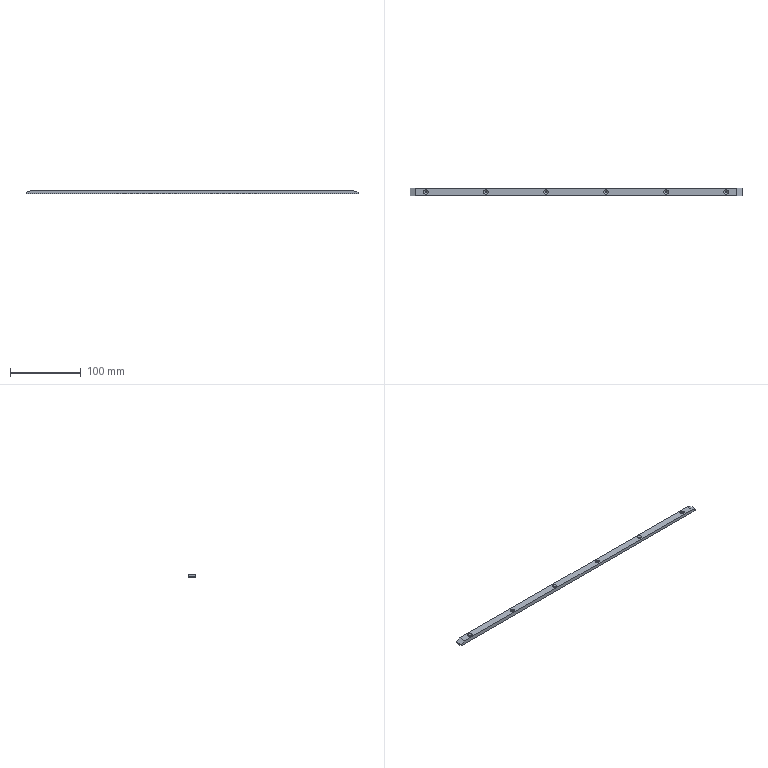Part | NX | features BREP 1 | 1 solid | 32 faces | box 470 x 10 x 5 mm | volume 22916 mm3 | cone 12 | cylinder 12 | plane 8 | commonest cylinder face diameters 3.4 x12
STEP:
#1=CARTESIAN_POINT('',(-215.65,0.,5.));
#2=VERTEX_POINT('',#1);
#3=CARTESIAN_POINT('',(-214.2,0.,3.55));
#4=VERTEX_POINT('',#3);
#5=CARTESIAN_POINT('',(-215.65,0.,5.));
#6=DIRECTION('',(-0.7071,0.,0.7071));
#7=VECTOR('',#6,1000.);
#8=LINE('',#5,#7);
#9=EDGE_CURVE('',#2,#4,#8,.F.);
#10=ORIENTED_EDGE('',*,*,#9,.T.);
#11=CARTESIAN_POINT('',(-210.8,0.,3.55));
#12=VERTEX_POINT('',#11);
#13=CARTESIAN_POINT('',(-212.5,0.,3.55));
#14=DIRECTION('',(0.,0.,1.));
#15=DIRECTION('',(1.,0.,0.));
#16=AXIS2_PLACEMENT_3D('',#13,#14,#15);
#17=CIRCLE('',#16,1.7);
#18=EDGE_CURVE('',#12,#4,#17,.T.);
#19=ORIENTED_EDGE('',*,*,#18,.F.);
#20=CARTESIAN_POINT('',(-209.35,0.,5.));
#21=VERTEX_POINT('',#20);
#22=CARTESIAN_POINT('',(-209.35,0.,5.));
#23=DIRECTION('',(0.7071,0.,0.7071));
#24=VECTOR('',#23,1000.);
#25=LINE('',#22,#24);
#26=EDGE_CURVE('',#21,#12,#25,.F.);
#27=ORIENTED_EDGE('',*,*,#26,.F.);
#28=CARTESIAN_POINT('',(-212.5,0.,5.));
#29=DIRECTION('',(0.,0.,1.));
#30=DIRECTION('',(1.,0.,0.));
#31=AXIS2_PLACEMENT_3D('',#28,#29,#30);
#32=CIRCLE('',#31,3.15);
#33=EDGE_CURVE('',#21,#2,#32,.T.);
#34=ORIENTED_EDGE('',*,*,#33,.T.);
#35=EDGE_LOOP('',(#10,#19,#27,#34));
#36=FACE_BOUND('',#35,.T.);
#37=CARTESIAN_POINT('',(-212.5,0.,5.));
#38=DIRECTION('',(0.,0.,1.));
#39=DIRECTION('',(1.,0.,0.));
#40=AXIS2_PLACEMENT_3D('',#37,#38,#39);
#41=CONICAL_SURFACE('',#40,3.15,0.7854);
#42=ADVANCED_FACE('',(#36),#41,.F.);
#43=CARTESIAN_POINT('',(-214.2,0.,0.));
#44=VERTEX_POINT('',#43);
#45=CARTESIAN_POINT('',(-214.2,0.,5.));
#46=DIRECTION('',(0.,0.,1.));
#47=VECTOR('',#46,1000.);
#48=LINE('',#45,#47);
#49=EDGE_CURVE('',#4,#44,#48,.F.);
#50=ORIENTED_EDGE('',*,*,#49,.T.);
#51=CARTESIAN_POINT('',(-210.8,0.,0.));
#52=VERTEX_POINT('',#51);
#53=CARTESIAN_POINT('',(-212.5,0.,0.));
#54=DIRECTION('',(0.,0.,1.));
#55=DIRECTION('',(1.,0.,0.));
#56=AXIS2_PLACEMENT_3D('',#53,#54,#55);
#57=CIRCLE('',#56,1.7);
#58=EDGE_CURVE('',#52,#44,#57,.T.);
#59=ORIENTED_EDGE('',*,*,#58,.F.);
#60=CARTESIAN_POINT('',(-210.8,0.,5.));
#61=DIRECTION('',(0.,0.,1.));
#62=VECTOR('',#61,1000.);
#63=LINE('',#60,#62);
#64=EDGE_CURVE('',#12,#52,#63,.F.);
#65=ORIENTED_EDGE('',*,*,#64,.F.);
#66=ORIENTED_EDGE('',*,*,#18,.T.);
#67=EDGE_LOOP('',(#50,#59,#65,#66));
#68=FACE_BOUND('',#67,.T.);
#69=CARTESIAN_POINT('',(-212.5,0.,5.));
#70=DIRECTION('',(0.,0.,1.));
#71=DIRECTION('',(1.,0.,0.));
#72=AXIS2_PLACEMENT_3D('',#69,#70,#71);
#73=CYLINDRICAL_SURFACE('',#72,1.7);
#74=ADVANCED_FACE('',(#68),#73,.F.);
#75=CARTESIAN_POINT('',(-130.65,0.,5.));
#76=VERTEX_POINT('',#75);
#77=CARTESIAN_POINT('',(-129.2,0.,3.55));
#78=VERTEX_POINT('',#77);
#79=CARTESIAN_POINT('',(-130.65,0.,5.));
#80=DIRECTION('',(-0.7071,0.,0.7071));
#81=VECTOR('',#80,1000.);
#82=LINE('',#79,#81);
#83=EDGE_CURVE('',#76,#78,#82,.F.);
#84=ORIENTED_EDGE('',*,*,#83,.T.);
#85=CARTESIAN_POINT('',(-125.8,0.,3.55));
#86=VERTEX_POINT('',#85);
#87=CARTESIAN_POINT('',(-127.5,0.,3.55));
#88=DIRECTION('',(0.,0.,1.));
#89=DIRECTION('',(1.,0.,0.));
#90=AXIS2_PLACEMENT_3D('',#87,#88,#89);
#91=CIRCLE('',#90,1.7);
#92=EDGE_CURVE('',#86,#78,#91,.T.);
#93=ORIENTED_EDGE('',*,*,#92,.F.);
#94=CARTESIAN_POINT('',(-124.35,0.,5.));
#95=VERTEX_POINT('',#94);
#96=CARTESIAN_POINT('',(-124.35,0.,5.));
#97=DIRECTION('',(0.7071,0.,0.7071));
#98=VECTOR('',#97,1000.);
#99=LINE('',#96,#98);
#100=EDGE_CURVE('',#95,#86,#99,.F.);
#101=ORIENTED_EDGE('',*,*,#100,.F.);
#102=CARTESIAN_POINT('',(-127.5,0.,5.));
#103=DIRECTION('',(0.,0.,1.));
#104=DIRECTION('',(1.,0.,0.));
#105=AXIS2_PLACEMENT_3D('',#102,#103,#104);
#106=CIRCLE('',#105,3.15);
#107=EDGE_CURVE('',#95,#76,#106,.T.);
#108=ORIENTED_EDGE('',*,*,#107,.T.);
#109=EDGE_LOOP('',(#84,#93,#101,#108));
#110=FACE_BOUND('',#109,.T.);
#111=CARTESIAN_POINT('',(-127.5,0.,5.));
#112=DIRECTION('',(0.,0.,1.));
#113=DIRECTION('',(1.,0.,0.));
#114=AXIS2_PLACEMENT_3D('',#111,#112,#113);
#115=CONICAL_SURFACE('',#114,3.15,0.7854);
#116=ADVANCED_FACE('',(#110),#115,.F.);
#117=CARTESIAN_POINT('',(-129.2,0.,0.));
#118=VERTEX_POINT('',#117);
#119=CARTESIAN_POINT('',(-129.2,0.,5.));
#120=DIRECTION('',(0.,0.,1.));
#121=VECTOR('',#120,1000.);
#122=LINE('',#119,#121);
#123=EDGE_CURVE('',#78,#118,#122,.F.);
#124=ORIENTED_EDGE('',*,*,#123,.T.);
#125=CARTESIAN_POINT('',(-125.8,0.,0.));
#126=VERTEX_POINT('',#125);
#127=CARTESIAN_POINT('',(-127.5,0.,0.));
#128=DIRECTION('',(0.,0.,1.));
#129=DIRECTION('',(1.,0.,0.));
#130=AXIS2_PLACEMENT_3D('',#127,#128,#129);
#131=CIRCLE('',#130,1.7);
#132=EDGE_CURVE('',#126,#118,#131,.T.);
#133=ORIENTED_EDGE('',*,*,#132,.F.);
#134=CARTESIAN_POINT('',(-125.8,0.,5.));
#135=DIRECTION('',(0.,0.,1.));
#136=VECTOR('',#135,1000.);
#137=LINE('',#134,#136);
#138=EDGE_CURVE('',#86,#126,#137,.F.);
#139=ORIENTED_EDGE('',*,*,#138,.F.);
#140=ORIENTED_EDGE('',*,*,#92,.T.);
#141=EDGE_LOOP('',(#124,#133,#139,#140));
#142=FACE_BOUND('',#141,.T.);
#143=CARTESIAN_POINT('',(-127.5,0.,5.));
#144=DIRECTION('',(0.,0.,1.));
#145=DIRECTION('',(1.,0.,0.));
#146=AXIS2_PLACEMENT_3D('',#143,#144,#145);
#147=CYLINDRICAL_SURFACE('',#146,1.7);
#148=ADVANCED_FACE('',(#142),#147,.F.);
#149=CARTESIAN_POINT('',(-45.65,0.,5.));
#150=VERTEX_POINT('',#149);
#151=CARTESIAN_POINT('',(-44.2,0.,3.55));
#152=VERTEX_POINT('',#151);
#153=CARTESIAN_POINT('',(-45.65,0.,5.));
#154=DIRECTION('',(-0.7071,0.,0.7071));
#155=VECTOR('',#154,1000.);
#156=LINE('',#153,#155);
#157=EDGE_CURVE('',#150,#152,#156,.F.);
#158=ORIENTED_EDGE('',*,*,#157,.T.);
#159=CARTESIAN_POINT('',(-40.8,0.,3.55));
#160=VERTEX_POINT('',#159);
#161=CARTESIAN_POINT('',(-42.5,0.,3.55));
#162=DIRECTION('',(0.,0.,1.));
#163=DIRECTION('',(1.,0.,0.));
#164=AXIS2_PLACEMENT_3D('',#161,#162,#163);
#165=CIRCLE('',#164,1.7);
#166=EDGE_CURVE('',#160,#152,#165,.T.);
#167=ORIENTED_EDGE('',*,*,#166,.F.);
#168=CARTESIAN_POINT('',(-39.35,0.,5.));
#169=VERTEX_POINT('',#168);
#170=CARTESIAN_POINT('',(-39.35,0.,5.));
#171=DIRECTION('',(0.7071,0.,0.7071));
#172=VECTOR('',#171,1000.);
#173=LINE('',#170,#172);
#174=EDGE_CURVE('',#169,#160,#173,.F.);
#175=ORIENTED_EDGE('',*,*,#174,.F.);
#176=CARTESIAN_POINT('',(-42.5,0.,5.));
#177=DIRECTION('',(0.,0.,1.));
#178=DIRECTION('',(1.,0.,0.));
#179=AXIS2_PLACEMENT_3D('',#176,#177,#178);
#180=CIRCLE('',#179,3.15);
#181=EDGE_CURVE('',#169,#150,#180,.T.);
#182=ORIENTED_EDGE('',*,*,#181,.T.);
#183=EDGE_LOOP('',(#158,#167,#175,#182));
#184=FACE_BOUND('',#183,.T.);
#185=CARTESIAN_POINT('',(-42.5,0.,5.));
#186=DIRECTION('',(0.,0.,1.));
#187=DIRECTION('',(1.,0.,0.));
#188=AXIS2_PLACEMENT_3D('',#185,#186,#187);
#189=CONICAL_SURFACE('',#188,3.15,0.7854);
#190=ADVANCED_FACE('',(#184),#189,.F.);
#191=CARTESIAN_POINT('',(-44.2,0.,0.));
#192=VERTEX_POINT('',#191);
#193=CARTESIAN_POINT('',(-44.2,0.,5.));
#194=DIRECTION('',(0.,0.,1.));
#195=VECTOR('',#194,1000.);
#196=LINE('',#193,#195);
#197=EDGE_CURVE('',#152,#192,#196,.F.);
#198=ORIENTED_EDGE('',*,*,#197,.T.);
#199=CARTESIAN_POINT('',(-40.8,0.,0.));
#200=VERTEX_POINT('',#199);
#201=CARTESIAN_POINT('',(-42.5,0.,0.));
#202=DIRECTION('',(0.,0.,1.));
#203=DIRECTION('',(1.,0.,0.));
#204=AXIS2_PLACEMENT_3D('',#201,#202,#203);
#205=CIRCLE('',#204,1.7);
#206=EDGE_CURVE('',#200,#192,#205,.T.);
#207=ORIENTED_EDGE('',*,*,#206,.F.);
#208=CARTESIAN_POINT('',(-40.8,0.,5.));
#209=DIRECTION('',(0.,0.,1.));
#210=VECTOR('',#209,1000.);
#211=LINE('',#208,#210);
#212=EDGE_CURVE('',#160,#200,#211,.F.);
#213=ORIENTED_EDGE('',*,*,#212,.F.);
#214=ORIENTED_EDGE('',*,*,#166,.T.);
#215=EDGE_LOOP('',(#198,#207,#213,#214));
#216=FACE_BOUND('',#215,.T.);
#217=CARTESIAN_POINT('',(-42.5,0.,5.));
#218=DIRECTION('',(0.,0.,1.));
#219=DIRECTION('',(1.,0.,0.));
#220=AXIS2_PLACEMENT_3D('',#217,#218,#219);
#221=CYLINDRICAL_SURFACE('',#220,1.7);
#222=ADVANCED_FACE('',(#216),#221,.F.);
#223=CARTESIAN_POINT('',(39.35,0.,5.));
#224=VERTEX_POINT('',#223);
#225=CARTESIAN_POINT('',(40.8,0.,3.55));
#226=VERTEX_POINT('',#225);
#227=CARTESIAN_POINT('',(39.35,0.,5.));
#228=DIRECTION('',(-0.7071,0.,0.7071));
#229=VECTOR('',#228,1000.);
#230=LINE('',#227,#229);
#231=EDGE_CURVE('',#224,#226,#230,.F.);
#232=ORIENTED_EDGE('',*,*,#231,.T.);
#233=CARTESIAN_POINT('',(44.2,0.,3.55));
#234=VERTEX_POINT('',#233);
#235=CARTESIAN_POINT('',(42.5,0.,3.55));
#236=DIRECTION('',(0.,0.,1.));
#237=DIRECTION('',(1.,0.,0.));
#238=AXIS2_PLACEMENT_3D('',#235,#236,#237);
#239=CIRCLE('',#238,1.7);
#240=EDGE_CURVE('',#234,#226,#239,.T.);
#241=ORIENTED_EDGE('',*,*,#240,.F.);
#242=CARTESIAN_POINT('',(45.65,0.,5.));
#243=VERTEX_POINT('',#242);
#244=CARTESIAN_POINT('',(45.65,0.,5.));
#245=DIRECTION('',(0.7071,0.,0.7071));
#246=VECTOR('',#245,1000.);
#247=LINE('',#244,#246);
#248=EDGE_CURVE('',#243,#234,#247,.F.);
#249=ORIENTED_EDGE('',*,*,#248,.F.);
#250=CARTESIAN_POINT('',(42.5,0.,5.));
#251=DIRECTION('',(0.,0.,1.));
#252=DIRECTION('',(1.,0.,0.));
#253=AXIS2_PLACEMENT_3D('',#250,#251,#252);
#254=CIRCLE('',#253,3.15);
#255=EDGE_CURVE('',#243,#224,#254,.T.);
#256=ORIENTED_EDGE('',*,*,#255,.T.);
#257=EDGE_LOOP('',(#232,#241,#249,#256));
#258=FACE_BOUND('',#257,.T.);
#259=CARTESIAN_POINT('',(42.5,0.,5.));
#260=DIRECTION('',(0.,0.,1.));
#261=DIRECTION('',(1.,0.,0.));
#262=AXIS2_PLACEMENT_3D('',#259,#260,#261);
#263=CONICAL_SURFACE('',#262,3.15,0.7854);
#264=ADVANCED_FACE('',(#258),#263,.F.);
#265=CARTESIAN_POINT('',(40.8,0.,0.));
#266=VERTEX_POINT('',#265);
#267=CARTESIAN_POINT('',(40.8,0.,5.));
#268=DIRECTION('',(0.,0.,1.));
#269=VECTOR('',#268,1000.);
#270=LINE('',#267,#269);
#271=EDGE_CURVE('',#226,#266,#270,.F.);
#272=ORIENTED_EDGE('',*,*,#271,.T.);
#273=CARTESIAN_POINT('',(44.2,0.,0.));
#274=VERTEX_POINT('',#273);
#275=CARTESIAN_POINT('',(42.5,0.,0.));
#276=DIRECTION('',(0.,0.,1.));
#277=DIRECTION('',(1.,0.,0.));
#278=AXIS2_PLACEMENT_3D('',#275,#276,#277);
#279=CIRCLE('',#278,1.7);
#280=EDGE_CURVE('',#274,#266,#279,.T.);
#281=ORIENTED_EDGE('',*,*,#280,.F.);
#282=CARTESIAN_POINT('',(44.2,0.,5.));
#283=DIRECTION('',(0.,0.,1.));
#284=VECTOR('',#283,1000.);
#285=LINE('',#282,#284);
#286=EDGE_CURVE('',#234,#274,#285,.F.);
#287=ORIENTED_EDGE('',*,*,#286,.F.);
#288=ORIENTED_EDGE('',*,*,#240,.T.);
#289=EDGE_LOOP('',(#272,#281,#287,#288));
#290=FACE_BOUND('',#289,.T.);
#291=CARTESIAN_POINT('',(42.5,0.,5.));
#292=DIRECTION('',(0.,0.,1.));
#293=DIRECTION('',(1.,0.,0.));
#294=AXIS2_PLACEMENT_3D('',#291,#292,#293);
#295=CYLINDRICAL_SURFACE('',#294,1.7);
#296=ADVANCED_FACE('',(#290),#295,.F.);
#297=CARTESIAN_POINT('',(124.35,0.,5.));
#298=VERTEX_POINT('',#297);
#299=CARTESIAN_POINT('',(125.8,0.,3.55));
#300=VERTEX_POINT('',#299);
#301=CARTESIAN_POINT('',(124.35,0.,5.));
#302=DIRECTION('',(-0.7071,0.,0.7071));
#303=VECTOR('',#302,1000.);
#304=LINE('',#301,#303);
#305=EDGE_CURVE('',#298,#300,#304,.F.);
#306=ORIENTED_EDGE('',*,*,#305,.T.);
#307=CARTESIAN_POINT('',(129.2,0.,3.55));
#308=VERTEX_POINT('',#307);
#309=CARTESIAN_POINT('',(127.5,0.,3.55));
#310=DIRECTION('',(0.,0.,1.));
#311=DIRECTION('',(1.,0.,0.));
#312=AXIS2_PLACEMENT_3D('',#309,#310,#311);
#313=CIRCLE('',#312,1.7);
#314=EDGE_CURVE('',#308,#300,#313,.T.);
#315=ORIENTED_EDGE('',*,*,#314,.F.);
#316=CARTESIAN_POINT('',(130.65,0.,5.));
#317=VERTEX_POINT('',#316);
#318=CARTESIAN_POINT('',(130.65,0.,5.));
#319=DIRECTION('',(0.7071,0.,0.7071));
#320=VECTOR('',#319,1000.);
#321=LINE('',#318,#320);
#322=EDGE_CURVE('',#317,#308,#321,.F.);
#323=ORIENTED_EDGE('',*,*,#322,.F.);
#324=CARTESIAN_POINT('',(127.5,0.,5.));
#325=DIRECTION('',(0.,0.,1.));
#326=DIRECTION('',(1.,0.,0.));
#327=AXIS2_PLACEMENT_3D('',#324,#325,#326);
#328=CIRCLE('',#327,3.15);
#329=EDGE_CURVE('',#317,#298,#328,.T.);
#330=ORIENTED_EDGE('',*,*,#329,.T.);
#331=EDGE_LOOP('',(#306,#315,#323,#330));
#332=FACE_BOUND('',#331,.T.);
#333=CARTESIAN_POINT('',(127.5,0.,5.));
#334=DIRECTION('',(0.,0.,1.));
#335=DIRECTION('',(1.,0.,0.));
#336=AXIS2_PLACEMENT_3D('',#333,#334,#335);
#337=CONICAL_SURFACE('',#336,3.15,0.7854);
#338=ADVANCED_FACE('',(#332),#337,.F.);
#339=CARTESIAN_POINT('',(125.8,0.,0.));
#340=VERTEX_POINT('',#339);
#341=CARTESIAN_POINT('',(125.8,0.,5.));
#342=DIRECTION('',(0.,0.,1.));
#343=VECTOR('',#342,1000.);
#344=LINE('',#341,#343);
#345=EDGE_CURVE('',#300,#340,#344,.F.);
#346=ORIENTED_EDGE('',*,*,#345,.T.);
#347=CARTESIAN_POINT('',(129.2,0.,0.));
#348=VERTEX_POINT('',#347);
#349=CARTESIAN_POINT('',(127.5,0.,0.));
#350=DIRECTION('',(0.,0.,1.));
#351=DIRECTION('',(1.,0.,0.));
#352=AXIS2_PLACEMENT_3D('',#349,#350,#351);
#353=CIRCLE('',#352,1.7);
#354=EDGE_CURVE('',#348,#340,#353,.T.);
#355=ORIENTED_EDGE('',*,*,#354,.F.);
#356=CARTESIAN_POINT('',(129.2,0.,5.));
#357=DIRECTION('',(0.,0.,1.));
#358=VECTOR('',#357,1000.);
#359=LINE('',#356,#358);
#360=EDGE_CURVE('',#308,#348,#359,.F.);
#361=ORIENTED_EDGE('',*,*,#360,.F.);
#362=ORIENTED_EDGE('',*,*,#314,.T.);
#363=EDGE_LOOP('',(#346,#355,#361,#362));
#364=FACE_BOUND('',#363,.T.);
#365=CARTESIAN_POINT('',(127.5,0.,5.));
#366=DIRECTION('',(0.,0.,1.));
#367=DIRECTION('',(1.,0.,0.));
#368=AXIS2_PLACEMENT_3D('',#365,#366,#367);
#369=CYLINDRICAL_SURFACE('',#368,1.7);
#370=ADVANCED_FACE('',(#364),#369,.F.);
#371=CARTESIAN_POINT('',(209.35,0.,5.));
#372=VERTEX_POINT('',#371);
#373=CARTESIAN_POINT('',(210.8,0.,3.55));
#374=VERTEX_POINT('',#373);
#375=CARTESIAN_POINT('',(209.35,0.,5.));
#376=DIRECTION('',(-0.7071,0.,0.7071));
#377=VECTOR('',#376,1000.);
#378=LINE('',#375,#377);
#379=EDGE_CURVE('',#372,#374,#378,.F.);
#380=ORIENTED_EDGE('',*,*,#379,.T.);
#381=CARTESIAN_POINT('',(214.2,0.,3.55));
#382=VERTEX_POINT('',#381);
#383=CARTESIAN_POINT('',(212.5,0.,3.55));
#384=DIRECTION('',(0.,0.,1.));
#385=DIRECTION('',(1.,0.,0.));
#386=AXIS2_PLACEMENT_3D('',#383,#384,#385);
#387=CIRCLE('',#386,1.7);
#388=EDGE_CURVE('',#382,#374,#387,.T.);
#389=ORIENTED_EDGE('',*,*,#388,.F.);
#390=CARTESIAN_POINT('',(215.65,0.,5.));
#391=VERTEX_POINT('',#390);
#392=CARTESIAN_POINT('',(215.65,0.,5.));
#393=DIRECTION('',(0.7071,0.,0.7071));
#394=VECTOR('',#393,1000.);
#395=LINE('',#392,#394);
#396=EDGE_CURVE('',#391,#382,#395,.F.);
#397=ORIENTED_EDGE('',*,*,#396,.F.);
#398=CARTESIAN_POINT('',(212.5,0.,5.));
#399=DIRECTION('',(0.,0.,1.));
#400=DIRECTION('',(1.,0.,0.));
#401=AXIS2_PLACEMENT_3D('',#398,#399,#400);
#402=CIRCLE('',#401,3.15);
#403=EDGE_CURVE('',#391,#372,#402,.T.);
#404=ORIENTED_EDGE('',*,*,#403,.T.);
#405=EDGE_LOOP('',(#380,#389,#397,#404));
#406=FACE_BOUND('',#405,.T.);
#407=CARTESIAN_POINT('',(212.5,0.,5.));
#408=DIRECTION('',(0.,0.,1.));
#409=DIRECTION('',(1.,0.,0.));
#410=AXIS2_PLACEMENT_3D('',#407,#408,#409);
#411=CONICAL_SURFACE('',#410,3.15,0.7854);
#412=ADVANCED_FACE('',(#406),#411,.F.);
#413=CARTESIAN_POINT('',(210.8,0.,0.));
#414=VERTEX_POINT('',#413);
#415=CARTESIAN_POINT('',(210.8,0.,5.));
#416=DIRECTION('',(0.,0.,1.));
#417=VECTOR('',#416,1000.);
#418=LINE('',#415,#417);
#419=EDGE_CURVE('',#374,#414,#418,.F.);
#420=ORIENTED_EDGE('',*,*,#419,.T.);
#421=CARTESIAN_POINT('',(214.2,0.,0.));
#422=VERTEX_POINT('',#421);
#423=CARTESIAN_POINT('',(212.5,0.,0.));
#424=DIRECTION('',(0.,0.,1.));
#425=DIRECTION('',(1.,0.,0.));
#426=AXIS2_PLACEMENT_3D('',#423,#424,#425);
#427=CIRCLE('',#426,1.7);
#428=EDGE_CURVE('',#422,#414,#427,.T.);
#429=ORIENTED_EDGE('',*,*,#428,.F.);
#430=CARTESIAN_POINT('',(214.2,0.,5.));
#431=DIRECTION('',(0.,0.,1.));
#432=VECTOR('',#431,1000.);
#433=LINE('',#430,#432);
#434=EDGE_CURVE('',#382,#422,#433,.F.);
#435=ORIENTED_EDGE('',*,*,#434,.F.);
#436=ORIENTED_EDGE('',*,*,#388,.T.);
#437=EDGE_LOOP('',(#420,#429,#435,#436));
#438=FACE_BOUND('',#437,.T.);
#439=CARTESIAN_POINT('',(212.5,0.,5.));
#440=DIRECTION('',(0.,0.,1.));
#441=DIRECTION('',(1.,0.,0.));
#442=AXIS2_PLACEMENT_3D('',#439,#440,#441);
#443=CYLINDRICAL_SURFACE('',#442,1.7);
#444=ADVANCED_FACE('',(#438),#443,.F.);
#445=CARTESIAN_POINT('',(-235.,5.,2.));
#446=VERTEX_POINT('',#445);
#447=CARTESIAN_POINT('',(-227.5,5.,5.));
#448=VERTEX_POINT('',#447);
#449=CARTESIAN_POINT('',(-227.5,5.,5.));
#450=DIRECTION('',(0.9285,0.,0.3714));
#451=VECTOR('',#450,1000.);
#452=LINE('',#449,#451);
#453=EDGE_CURVE('',#446,#448,#452,.T.);
#454=ORIENTED_EDGE('',*,*,#453,.F.);
#455=CARTESIAN_POINT('',(-235.,-5.,2.));
#456=VERTEX_POINT('',#455);
#457=CARTESIAN_POINT('',(-235.,-5.,2.));
#458=DIRECTION('',(0.,1.,0.));
#459=VECTOR('',#458,1000.);
#460=LINE('',#457,#459);
#461=EDGE_CURVE('',#456,#446,#460,.T.);
#462=ORIENTED_EDGE('',*,*,#461,.F.);
#463=CARTESIAN_POINT('',(-227.5,-5.,5.));
#464=VERTEX_POINT('',#463);
#465=CARTESIAN_POINT('',(-227.5,-5.,5.));
#466=DIRECTION('',(-0.9285,0.,-0.3714));
#467=VECTOR('',#466,1000.);
#468=LINE('',#465,#467);
#469=EDGE_CURVE('',#464,#456,#468,.T.);
#470=ORIENTED_EDGE('',*,*,#469,.F.);
#471=CARTESIAN_POINT('',(-227.5,0.,5.));
#472=DIRECTION('',(0.,-1.,0.));
#473=VECTOR('',#472,1000.);
#474=LINE('',#471,#473);
#475=EDGE_CURVE('',#448,#464,#474,.T.);
#476=ORIENTED_EDGE('',*,*,#475,.F.);
#477=EDGE_LOOP('',(#454,#462,#470,#476));
#478=FACE_BOUND('',#477,.T.);
#479=CARTESIAN_POINT('',(-227.5,0.,5.));
#480=DIRECTION('',(0.3714,0.,-0.9285));
#481=DIRECTION('',(0.,-1.,0.));
#482=AXIS2_PLACEMENT_3D('',#479,#480,#481);
#483=PLANE('',#482);
#484=ADVANCED_FACE('',(#478),#483,.F.);
#485=CARTESIAN_POINT('',(235.,-5.,2.));
#486=VERTEX_POINT('',#485);
#487=CARTESIAN_POINT('',(227.5,-5.,5.));
#488=VERTEX_POINT('',#487);
#489=CARTESIAN_POINT('',(227.5,-5.,5.));
#490=DIRECTION('',(-0.9285,0.,0.3714));
#491=VECTOR('',#490,1000.);
#492=LINE('',#489,#491);
#493=EDGE_CURVE('',#486,#488,#492,.T.);
#494=ORIENTED_EDGE('',*,*,#493,.F.);
#495=CARTESIAN_POINT('',(235.,5.,2.));
#496=VERTEX_POINT('',#495);
#497=CARTESIAN_POINT('',(235.,-5.,2.));
#498=DIRECTION('',(0.,-1.,0.));
#499=VECTOR('',#498,1000.);
#500=LINE('',#497,#499);
#501=EDGE_CURVE('',#496,#486,#500,.T.);
#502=ORIENTED_EDGE('',*,*,#501,.F.);
#503=CARTESIAN_POINT('',(227.5,5.,5.));
#504=VERTEX_POINT('',#503);
#505=CARTESIAN_POINT('',(227.5,5.,5.));
#506=DIRECTION('',(0.9285,0.,-0.3714));
#507=VECTOR('',#506,1000.);
#508=LINE('',#505,#507);
#509=EDGE_CURVE('',#504,#496,#508,.T.);
#510=ORIENTED_EDGE('',*,*,#509,.F.);
#511=CARTESIAN_POINT('',(227.5,0.,5.));
#512=DIRECTION('',(0.,1.,0.));
#513=VECTOR('',#512,1000.);
#514=LINE('',#511,#513);
#515=EDGE_CURVE('',#488,#504,#514,.T.);
#516=ORIENTED_EDGE('',*,*,#515,.F.);
#517=EDGE_LOOP('',(#494,#502,#510,#516));
#518=FACE_BOUND('',#517,.T.);
#519=CARTESIAN_POINT('',(227.5,0.,5.));
#520=DIRECTION('',(-0.3714,0.,-0.9285));
#521=DIRECTION('',(0.,1.,0.));
#522=AXIS2_PLACEMENT_3D('',#519,#520,#521);
#523=PLANE('',#522);
#524=ADVANCED_FACE('',(#518),#523,.F.);
#525=CARTESIAN_POINT('',(235.,-5.,0.));
#526=VERTEX_POINT('',#525);
#527=CARTESIAN_POINT('',(235.,5.,0.));
#528=VERTEX_POINT('',#527);
#529=CARTESIAN_POINT('',(235.,-5.,0.));
#530=DIRECTION('',(0.,1.,0.));
#531=VECTOR('',#530,1000.);
#532=LINE('',#529,#531);
#533=EDGE_CURVE('',#526,#528,#532,.T.);
#534=ORIENTED_EDGE('',*,*,#533,.F.);
#535=CARTESIAN_POINT('',(-235.,-5.,0.));
#536=VERTEX_POINT('',#535);
#537=CARTESIAN_POINT('',(-235.,-5.,0.));
#538=DIRECTION('',(1.,0.,0.));
#539=VECTOR('',#538,1000.);
#540=LINE('',#537,#539);
#541=EDGE_CURVE('',#536,#526,#540,.T.);
#542=ORIENTED_EDGE('',*,*,#541,.F.);
#543=CARTESIAN_POINT('',(-235.,5.,0.));
#544=VERTEX_POINT('',#543);
#545=CARTESIAN_POINT('',(-235.,-5.,0.));
#546=DIRECTION('',(0.,-1.,0.));
#547=VECTOR('',#546,1000.);
#548=LINE('',#545,#547);
#549=EDGE_CURVE('',#544,#536,#548,.T.);
#550=ORIENTED_EDGE('',*,*,#549,.F.);
#551=CARTESIAN_POINT('',(-235.,5.,0.));
#552=DIRECTION('',(-1.,0.,0.));
#553=VECTOR('',#552,1000.);
#554=LINE('',#551,#553);
#555=EDGE_CURVE('',#528,#544,#554,.T.);
#556=ORIENTED_EDGE('',*,*,#555,.F.);
#557=EDGE_LOOP('',(#534,#542,#550,#556));
#558=FACE_BOUND('',#557,.T.);
#559=ORIENTED_EDGE('',*,*,#428,.T.);
#560=CARTESIAN_POINT('',(212.5,0.,0.));
#561=DIRECTION('',(0.,0.,1.));
#562=DIRECTION('',(1.,0.,0.));
#563=AXIS2_PLACEMENT_3D('',#560,#561,#562);
#564=CIRCLE('',#563,1.7);
#565=EDGE_CURVE('',#414,#422,#564,.T.);
#566=ORIENTED_EDGE('',*,*,#565,.T.);
#567=EDGE_LOOP('',(#559,#566));
#568=FACE_BOUND('',#567,.T.);
#569=ORIENTED_EDGE('',*,*,#354,.T.);
#570=CARTESIAN_POINT('',(127.5,0.,0.));
#571=DIRECTION('',(0.,0.,1.));
#572=DIRECTION('',(1.,0.,0.));
#573=AXIS2_PLACEMENT_3D('',#570,#571,#572);
#574=CIRCLE('',#573,1.7);
#575=EDGE_CURVE('',#340,#348,#574,.T.);
#576=ORIENTED_EDGE('',*,*,#575,.T.);
#577=EDGE_LOOP('',(#569,#576));
#578=FACE_BOUND('',#577,.T.);
#579=ORIENTED_EDGE('',*,*,#280,.T.);
#580=CARTESIAN_POINT('',(42.5,0.,0.));
#581=DIRECTION('',(0.,0.,1.));
#582=DIRECTION('',(1.,0.,0.));
#583=AXIS2_PLACEMENT_3D('',#580,#581,#582);
#584=CIRCLE('',#583,1.7);
#585=EDGE_CURVE('',#266,#274,#584,.T.);
#586=ORIENTED_EDGE('',*,*,#585,.T.);
#587=EDGE_LOOP('',(#579,#586));
#588=FACE_BOUND('',#587,.T.);
#589=ORIENTED_EDGE('',*,*,#206,.T.);
#590=CARTESIAN_POINT('',(-42.5,0.,0.));
#591=DIRECTION('',(0.,0.,1.));
#592=DIRECTION('',(1.,0.,0.));
#593=AXIS2_PLACEMENT_3D('',#590,#591,#592);
#594=CIRCLE('',#593,1.7);
#595=EDGE_CURVE('',#192,#200,#594,.T.);
#596=ORIENTED_EDGE('',*,*,#595,.T.);
#597=EDGE_LOOP('',(#589,#596));
#598=FACE_BOUND('',#597,.T.);
#599=ORIENTED_EDGE('',*,*,#132,.T.);
#600=CARTESIAN_POINT('',(-127.5,0.,0.));
#601=DIRECTION('',(0.,0.,1.));
#602=DIRECTION('',(1.,0.,0.));
#603=AXIS2_PLACEMENT_3D('',#600,#601,#602);
#604=CIRCLE('',#603,1.7);
#605=EDGE_CURVE('',#118,#126,#604,.T.);
#606=ORIENTED_EDGE('',*,*,#605,.T.);
#607=EDGE_LOOP('',(#599,#606));
#608=FACE_BOUND('',#607,.T.);
#609=ORIENTED_EDGE('',*,*,#58,.T.);
#610=CARTESIAN_POINT('',(-212.5,0.,0.));
#611=DIRECTION('',(0.,0.,1.));
#612=DIRECTION('',(1.,0.,0.));
#613=AXIS2_PLACEMENT_3D('',#610,#611,#612);
#614=CIRCLE('',#613,1.7);
#615=EDGE_CURVE('',#44,#52,#614,.T.);
#616=ORIENTED_EDGE('',*,*,#615,.T.);
#617=EDGE_LOOP('',(#609,#616));
#618=FACE_BOUND('',#617,.T.);
#619=CARTESIAN_POINT('',(0.,0.,0.));
#620=DIRECTION('',(0.,0.,-1.));
#621=DIRECTION('',(-1.,0.,0.));
#622=AXIS2_PLACEMENT_3D('',#619,#620,#621);
#623=PLANE('',#622);
#624=ADVANCED_FACE('',(#558,#568,#578,#588,#598,#608,#618),#623,.T.);
#625=CARTESIAN_POINT('',(-235.,-5.,5.));
#626=DIRECTION('',(1.,0.,0.));
#627=VECTOR('',#626,1000.);
#628=LINE('',#625,#627);
#629=EDGE_CURVE('',#464,#488,#628,.T.);
#630=ORIENTED_EDGE('',*,*,#629,.T.);
#631=ORIENTED_EDGE('',*,*,#515,.T.);
#632=CARTESIAN_POINT('',(-235.,5.,5.));
#633=DIRECTION('',(-1.,0.,0.));
#634=VECTOR('',#633,1000.);
#635=LINE('',#632,#634);
#636=EDGE_CURVE('',#504,#448,#635,.T.);
#637=ORIENTED_EDGE('',*,*,#636,.T.);
#638=ORIENTED_EDGE('',*,*,#475,.T.);
#639=EDGE_LOOP('',(#630,#631,#637,#638));
#640=FACE_BOUND('',#639,.T.);
#641=ORIENTED_EDGE('',*,*,#403,.F.);
#642=CARTESIAN_POINT('',(212.5,0.,5.));
#643=DIRECTION('',(0.,0.,1.));
#644=DIRECTION('',(1.,0.,0.));
#645=AXIS2_PLACEMENT_3D('',#642,#643,#644);
#646=CIRCLE('',#645,3.15);
#647=EDGE_CURVE('',#372,#391,#646,.T.);
#648=ORIENTED_EDGE('',*,*,#647,.F.);
#649=EDGE_LOOP('',(#641,#648));
#650=FACE_BOUND('',#649,.T.);
#651=ORIENTED_EDGE('',*,*,#329,.F.);
#652=CARTESIAN_POINT('',(127.5,0.,5.));
#653=DIRECTION('',(0.,0.,1.));
#654=DIRECTION('',(1.,0.,0.));
#655=AXIS2_PLACEMENT_3D('',#652,#653,#654);
#656=CIRCLE('',#655,3.15);
#657=EDGE_CURVE('',#298,#317,#656,.T.);
#658=ORIENTED_EDGE('',*,*,#657,.F.);
#659=EDGE_LOOP('',(#651,#658));
#660=FACE_BOUND('',#659,.T.);
#661=ORIENTED_EDGE('',*,*,#255,.F.);
#662=CARTESIAN_POINT('',(42.5,0.,5.));
#663=DIRECTION('',(0.,0.,1.));
#664=DIRECTION('',(1.,0.,0.));
#665=AXIS2_PLACEMENT_3D('',#662,#663,#664);
#666=CIRCLE('',#665,3.15);
#667=EDGE_CURVE('',#224,#243,#666,.T.);
#668=ORIENTED_EDGE('',*,*,#667,.F.);
#669=EDGE_LOOP('',(#661,#668));
#670=FACE_BOUND('',#669,.T.);
#671=ORIENTED_EDGE('',*,*,#181,.F.);
#672=CARTESIAN_POINT('',(-42.5,0.,5.));
#673=DIRECTION('',(0.,0.,1.));
#674=DIRECTION('',(1.,0.,0.));
#675=AXIS2_PLACEMENT_3D('',#672,#673,#674);
#676=CIRCLE('',#675,3.15);
#677=EDGE_CURVE('',#150,#169,#676,.T.);
#678=ORIENTED_EDGE('',*,*,#677,.F.);
#679=EDGE_LOOP('',(#671,#678));
#680=FACE_BOUND('',#679,.T.);
#681=ORIENTED_EDGE('',*,*,#107,.F.);
#682=CARTESIAN_POINT('',(-127.5,0.,5.));
#683=DIRECTION('',(0.,0.,1.));
#684=DIRECTION('',(1.,0.,0.));
#685=AXIS2_PLACEMENT_3D('',#682,#683,#684);
#686=CIRCLE('',#685,3.15);
#687=EDGE_CURVE('',#76,#95,#686,.T.);
#688=ORIENTED_EDGE('',*,*,#687,.F.);
#689=EDGE_LOOP('',(#681,#688));
#690=FACE_BOUND('',#689,.T.);
#691=ORIENTED_EDGE('',*,*,#33,.F.);
#692=CARTESIAN_POINT('',(-212.5,0.,5.));
#693=DIRECTION('',(0.,0.,1.));
#694=DIRECTION('',(1.,0.,0.));
#695=AXIS2_PLACEMENT_3D('',#692,#693,#694);
#696=CIRCLE('',#695,3.15);
#697=EDGE_CURVE('',#2,#21,#696,.T.);
#698=ORIENTED_EDGE('',*,*,#697,.F.);
#699=EDGE_LOOP('',(#691,#698));
#700=FACE_BOUND('',#699,.T.);
#701=CARTESIAN_POINT('',(0.,0.,5.));
#702=DIRECTION('',(0.,0.,-1.));
#703=DIRECTION('',(-1.,0.,0.));
#704=AXIS2_PLACEMENT_3D('',#701,#702,#703);
#705=PLANE('',#704);
#706=ADVANCED_FACE('',(#640,#650,#660,#670,#680,#690,#700),#705,.F.);
#707=CARTESIAN_POINT('',(235.,-5.,5.));
#708=DIRECTION('',(0.,0.,-1.));
#709=VECTOR('',#708,1000.);
#710=LINE('',#707,#709);
#711=EDGE_CURVE('',#486,#526,#710,.T.);
#712=ORIENTED_EDGE('',*,*,#711,.F.);
#713=ORIENTED_EDGE('',*,*,#493,.T.);
#714=ORIENTED_EDGE('',*,*,#629,.F.);
#715=ORIENTED_EDGE('',*,*,#469,.T.);
#716=CARTESIAN_POINT('',(-235.,-5.,5.));
#717=DIRECTION('',(0.,0.,-1.));
#718=VECTOR('',#717,1000.);
#719=LINE('',#716,#718);
#720=EDGE_CURVE('',#456,#536,#719,.T.);
#721=ORIENTED_EDGE('',*,*,#720,.T.);
#722=ORIENTED_EDGE('',*,*,#541,.T.);
#723=EDGE_LOOP('',(#712,#713,#714,#715,#721,#722));
#724=FACE_BOUND('',#723,.T.);
#725=CARTESIAN_POINT('',(-235.,-5.,5.));
#726=DIRECTION('',(0.,1.,0.));
#727=DIRECTION('',(0.,0.,1.));
#728=AXIS2_PLACEMENT_3D('',#725,#726,#727);
#729=PLANE('',#728);
#730=ADVANCED_FACE('',(#724),#729,.F.);
#731=ORIENTED_EDGE('',*,*,#720,.F.);
#732=ORIENTED_EDGE('',*,*,#461,.T.);
#733=CARTESIAN_POINT('',(-235.,5.,5.));
#734=DIRECTION('',(0.,0.,-1.));
#735=VECTOR('',#734,1000.);
#736=LINE('',#733,#735);
#737=EDGE_CURVE('',#446,#544,#736,.T.);
#738=ORIENTED_EDGE('',*,*,#737,.T.);
#739=ORIENTED_EDGE('',*,*,#549,.T.);
#740=EDGE_LOOP('',(#731,#732,#738,#739));
#741=FACE_BOUND('',#740,.T.);
#742=CARTESIAN_POINT('',(-235.,-5.,5.));
#743=DIRECTION('',(1.,0.,0.));
#744=DIRECTION('',(0.,0.,-1.));
#745=AXIS2_PLACEMENT_3D('',#742,#743,#744);
#746=PLANE('',#745);
#747=ADVANCED_FACE('',(#741),#746,.F.);
#748=ORIENTED_EDGE('',*,*,#636,.F.);
#749=ORIENTED_EDGE('',*,*,#509,.T.);
#750=CARTESIAN_POINT('',(235.,5.,5.));
#751=DIRECTION('',(0.,0.,-1.));
#752=VECTOR('',#751,1000.);
#753=LINE('',#750,#752);
#754=EDGE_CURVE('',#496,#528,#753,.T.);
#755=ORIENTED_EDGE('',*,*,#754,.T.);
#756=ORIENTED_EDGE('',*,*,#555,.T.);
#757=ORIENTED_EDGE('',*,*,#737,.F.);
#758=ORIENTED_EDGE('',*,*,#453,.T.);
#759=EDGE_LOOP('',(#748,#749,#755,#756,#757,#758));
#760=FACE_BOUND('',#759,.T.);
#761=CARTESIAN_POINT('',(-235.,5.,5.));
#762=DIRECTION('',(0.,-1.,0.));
#763=DIRECTION('',(0.,0.,-1.));
#764=AXIS2_PLACEMENT_3D('',#761,#762,#763);
#765=PLANE('',#764);
#766=ADVANCED_FACE('',(#760),#765,.F.);
#767=ORIENTED_EDGE('',*,*,#754,.F.);
#768=ORIENTED_EDGE('',*,*,#501,.T.);
#769=ORIENTED_EDGE('',*,*,#711,.T.);
#770=ORIENTED_EDGE('',*,*,#533,.T.);
#771=EDGE_LOOP('',(#767,#768,#769,#770));
#772=FACE_BOUND('',#771,.T.);
#773=CARTESIAN_POINT('',(235.,-5.,5.));
#774=DIRECTION('',(-1.,0.,0.));
#775=DIRECTION('',(0.,0.,1.));
#776=AXIS2_PLACEMENT_3D('',#773,#774,#775);
#777=PLANE('',#776);
#778=ADVANCED_FACE('',(#772),#777,.F.);
#779=ORIENTED_EDGE('',*,*,#565,.F.);
#780=ORIENTED_EDGE('',*,*,#419,.F.);
#781=CARTESIAN_POINT('',(212.5,0.,3.55));
#782=DIRECTION('',(0.,0.,1.));
#783=DIRECTION('',(1.,0.,0.));
#784=AXIS2_PLACEMENT_3D('',#781,#782,#783);
#785=CIRCLE('',#784,1.7);
#786=EDGE_CURVE('',#374,#382,#785,.T.);
#787=ORIENTED_EDGE('',*,*,#786,.T.);
#788=ORIENTED_EDGE('',*,*,#434,.T.);
#789=EDGE_LOOP('',(#779,#780,#787,#788));
#790=FACE_BOUND('',#789,.T.);
#791=CARTESIAN_POINT('',(212.5,0.,5.));
#792=DIRECTION('',(0.,0.,1.));
#793=DIRECTION('',(1.,0.,0.));
#794=AXIS2_PLACEMENT_3D('',#791,#792,#793);
#795=CYLINDRICAL_SURFACE('',#794,1.7);
#796=ADVANCED_FACE('',(#790),#795,.F.);
#797=ORIENTED_EDGE('',*,*,#786,.F.);
#798=ORIENTED_EDGE('',*,*,#379,.F.);
#799=ORIENTED_EDGE('',*,*,#647,.T.);
#800=ORIENTED_EDGE('',*,*,#396,.T.);
#801=EDGE_LOOP('',(#797,#798,#799,#800));
#802=FACE_BOUND('',#801,.T.);
#803=CARTESIAN_POINT('',(212.5,0.,5.));
#804=DIRECTION('',(0.,0.,1.));
#805=DIRECTION('',(1.,0.,0.));
#806=AXIS2_PLACEMENT_3D('',#803,#804,#805);
#807=CONICAL_SURFACE('',#806,3.15,0.7854);
#808=ADVANCED_FACE('',(#802),#807,.F.);
#809=ORIENTED_EDGE('',*,*,#575,.F.);
#810=ORIENTED_EDGE('',*,*,#345,.F.);
#811=CARTESIAN_POINT('',(127.5,0.,3.55));
#812=DIRECTION('',(0.,0.,1.));
#813=DIRECTION('',(1.,0.,0.));
#814=AXIS2_PLACEMENT_3D('',#811,#812,#813);
#815=CIRCLE('',#814,1.7);
#816=EDGE_CURVE('',#300,#308,#815,.T.);
#817=ORIENTED_EDGE('',*,*,#816,.T.);
#818=ORIENTED_EDGE('',*,*,#360,.T.);
#819=EDGE_LOOP('',(#809,#810,#817,#818));
#820=FACE_BOUND('',#819,.T.);
#821=CARTESIAN_POINT('',(127.5,0.,5.));
#822=DIRECTION('',(0.,0.,1.));
#823=DIRECTION('',(1.,0.,0.));
#824=AXIS2_PLACEMENT_3D('',#821,#822,#823);
#825=CYLINDRICAL_SURFACE('',#824,1.7);
#826=ADVANCED_FACE('',(#820),#825,.F.);
#827=ORIENTED_EDGE('',*,*,#816,.F.);
#828=ORIENTED_EDGE('',*,*,#305,.F.);
#829=ORIENTED_EDGE('',*,*,#657,.T.);
#830=ORIENTED_EDGE('',*,*,#322,.T.);
#831=EDGE_LOOP('',(#827,#828,#829,#830));
#832=FACE_BOUND('',#831,.T.);
#833=CARTESIAN_POINT('',(127.5,0.,5.));
#834=DIRECTION('',(0.,0.,1.));
#835=DIRECTION('',(1.,0.,0.));
#836=AXIS2_PLACEMENT_3D('',#833,#834,#835);
#837=CONICAL_SURFACE('',#836,3.15,0.7854);
#838=ADVANCED_FACE('',(#832),#837,.F.);
#839=ORIENTED_EDGE('',*,*,#585,.F.);
#840=ORIENTED_EDGE('',*,*,#271,.F.);
#841=CARTESIAN_POINT('',(42.5,0.,3.55));
#842=DIRECTION('',(0.,0.,1.));
#843=DIRECTION('',(1.,0.,0.));
#844=AXIS2_PLACEMENT_3D('',#841,#842,#843);
#845=CIRCLE('',#844,1.7);
#846=EDGE_CURVE('',#226,#234,#845,.T.);
#847=ORIENTED_EDGE('',*,*,#846,.T.);
#848=ORIENTED_EDGE('',*,*,#286,.T.);
#849=EDGE_LOOP('',(#839,#840,#847,#848));
#850=FACE_BOUND('',#849,.T.);
#851=CARTESIAN_POINT('',(42.5,0.,5.));
#852=DIRECTION('',(0.,0.,1.));
#853=DIRECTION('',(1.,0.,0.));
#854=AXIS2_PLACEMENT_3D('',#851,#852,#853);
#855=CYLINDRICAL_SURFACE('',#854,1.7);
#856=ADVANCED_FACE('',(#850),#855,.F.);
#857=ORIENTED_EDGE('',*,*,#846,.F.);
#858=ORIENTED_EDGE('',*,*,#231,.F.);
#859=ORIENTED_EDGE('',*,*,#667,.T.);
#860=ORIENTED_EDGE('',*,*,#248,.T.);
#861=EDGE_LOOP('',(#857,#858,#859,#860));
#862=FACE_BOUND('',#861,.T.);
#863=CARTESIAN_POINT('',(42.5,0.,5.));
#864=DIRECTION('',(0.,0.,1.));
#865=DIRECTION('',(1.,0.,0.));
#866=AXIS2_PLACEMENT_3D('',#863,#864,#865);
#867=CONICAL_SURFACE('',#866,3.15,0.7854);
#868=ADVANCED_FACE('',(#862),#867,.F.);
#869=ORIENTED_EDGE('',*,*,#595,.F.);
#870=ORIENTED_EDGE('',*,*,#197,.F.);
#871=CARTESIAN_POINT('',(-42.5,0.,3.55));
#872=DIRECTION('',(0.,0.,1.));
#873=DIRECTION('',(1.,0.,0.));
#874=AXIS2_PLACEMENT_3D('',#871,#872,#873);
#875=CIRCLE('',#874,1.7);
#876=EDGE_CURVE('',#152,#160,#875,.T.);
#877=ORIENTED_EDGE('',*,*,#876,.T.);
#878=ORIENTED_EDGE('',*,*,#212,.T.);
#879=EDGE_LOOP('',(#869,#870,#877,#878));
#880=FACE_BOUND('',#879,.T.);
#881=CARTESIAN_POINT('',(-42.5,0.,5.));
#882=DIRECTION('',(0.,0.,1.));
#883=DIRECTION('',(1.,0.,0.));
#884=AXIS2_PLACEMENT_3D('',#881,#882,#883);
#885=CYLINDRICAL_SURFACE('',#884,1.7);
#886=ADVANCED_FACE('',(#880),#885,.F.);
#887=ORIENTED_EDGE('',*,*,#876,.F.);
#888=ORIENTED_EDGE('',*,*,#157,.F.);
#889=ORIENTED_EDGE('',*,*,#677,.T.);
#890=ORIENTED_EDGE('',*,*,#174,.T.);
#891=EDGE_LOOP('',(#887,#888,#889,#890));
#892=FACE_BOUND('',#891,.T.);
#893=CARTESIAN_POINT('',(-42.5,0.,5.));
#894=DIRECTION('',(0.,0.,1.));
#895=DIRECTION('',(1.,0.,0.));
#896=AXIS2_PLACEMENT_3D('',#893,#894,#895);
#897=CONICAL_SURFACE('',#896,3.15,0.7854);
#898=ADVANCED_FACE('',(#892),#897,.F.);
#899=ORIENTED_EDGE('',*,*,#605,.F.);
#900=ORIENTED_EDGE('',*,*,#123,.F.);
#901=CARTESIAN_POINT('',(-127.5,0.,3.55));
#902=DIRECTION('',(0.,0.,1.));
#903=DIRECTION('',(1.,0.,0.));
#904=AXIS2_PLACEMENT_3D('',#901,#902,#903);
#905=CIRCLE('',#904,1.7);
#906=EDGE_CURVE('',#78,#86,#905,.T.);
#907=ORIENTED_EDGE('',*,*,#906,.T.);
#908=ORIENTED_EDGE('',*,*,#138,.T.);
#909=EDGE_LOOP('',(#899,#900,#907,#908));
#910=FACE_BOUND('',#909,.T.);
#911=CARTESIAN_POINT('',(-127.5,0.,5.));
#912=DIRECTION('',(0.,0.,1.));
#913=DIRECTION('',(1.,0.,0.));
#914=AXIS2_PLACEMENT_3D('',#911,#912,#913);
#915=CYLINDRICAL_SURFACE('',#914,1.7);
#916=ADVANCED_FACE('',(#910),#915,.F.);
#917=ORIENTED_EDGE('',*,*,#906,.F.);
#918=ORIENTED_EDGE('',*,*,#83,.F.);
#919=ORIENTED_EDGE('',*,*,#687,.T.);
#920=ORIENTED_EDGE('',*,*,#100,.T.);
#921=EDGE_LOOP('',(#917,#918,#919,#920));
#922=FACE_BOUND('',#921,.T.);
#923=CARTESIAN_POINT('',(-127.5,0.,5.));
#924=DIRECTION('',(0.,0.,1.));
#925=DIRECTION('',(1.,0.,0.));
#926=AXIS2_PLACEMENT_3D('',#923,#924,#925);
#927=CONICAL_SURFACE('',#926,3.15,0.7854);
#928=ADVANCED_FACE('',(#922),#927,.F.);
#929=ORIENTED_EDGE('',*,*,#615,.F.);
#930=ORIENTED_EDGE('',*,*,#49,.F.);
#931=CARTESIAN_POINT('',(-212.5,0.,3.55));
#932=DIRECTION('',(0.,0.,1.));
#933=DIRECTION('',(1.,0.,0.));
#934=AXIS2_PLACEMENT_3D('',#931,#932,#933);
#935=CIRCLE('',#934,1.7);
#936=EDGE_CURVE('',#4,#12,#935,.T.);
#937=ORIENTED_EDGE('',*,*,#936,.T.);
#938=ORIENTED_EDGE('',*,*,#64,.T.);
#939=EDGE_LOOP('',(#929,#930,#937,#938));
#940=FACE_BOUND('',#939,.T.);
#941=CARTESIAN_POINT('',(-212.5,0.,5.));
#942=DIRECTION('',(0.,0.,1.));
#943=DIRECTION('',(1.,0.,0.));
#944=AXIS2_PLACEMENT_3D('',#941,#942,#943);
#945=CYLINDRICAL_SURFACE('',#944,1.7);
#946=ADVANCED_FACE('',(#940),#945,.F.);
#947=ORIENTED_EDGE('',*,*,#936,.F.);
#948=ORIENTED_EDGE('',*,*,#9,.F.);
#949=ORIENTED_EDGE('',*,*,#697,.T.);
#950=ORIENTED_EDGE('',*,*,#26,.T.);
#951=EDGE_LOOP('',(#947,#948,#949,#950));
#952=FACE_BOUND('',#951,.T.);
#953=CARTESIAN_POINT('',(-212.5,0.,5.));
#954=DIRECTION('',(0.,0.,1.));
#955=DIRECTION('',(1.,0.,0.));
#956=AXIS2_PLACEMENT_3D('',#953,#954,#955);
#957=CONICAL_SURFACE('',#956,3.15,0.7854);
#958=ADVANCED_FACE('',(#952),#957,.F.);
#959=CLOSED_SHELL('',(#42,#74,#116,#148,#190,#222,#264,#296,#338,#370,#412,#444,#484,#524,#624,#706,#730,#747,#766,#778,#796,#808,#826,#838,#856,#868,#886,#898,#916,#928,#946,#958));
#960=MANIFOLD_SOLID_BREP('',#959);
#961=(LENGTH_UNIT()NAMED_UNIT(*)SI_UNIT(.MILLI.,.METRE.));
#962=UNCERTAINTY_MEASURE_WITH_UNIT(LENGTH_MEASURE(0.00001),#961,'','');
#963=(NAMED_UNIT(*)PLANE_ANGLE_UNIT()SI_UNIT($,.RADIAN.));
#964=(NAMED_UNIT(*)SI_UNIT($,.STERADIAN.)SOLID_ANGLE_UNIT());
#965=(GEOMETRIC_REPRESENTATION_CONTEXT(3)GLOBAL_UNCERTAINTY_ASSIGNED_CONTEXT((#962))GLOBAL_UNIT_ASSIGNED_CONTEXT((#961,#963,#964))REPRESENTATION_CONTEXT('',''));
#966=ADVANCED_BREP_SHAPE_REPRESENTATION('',(#960),#965);